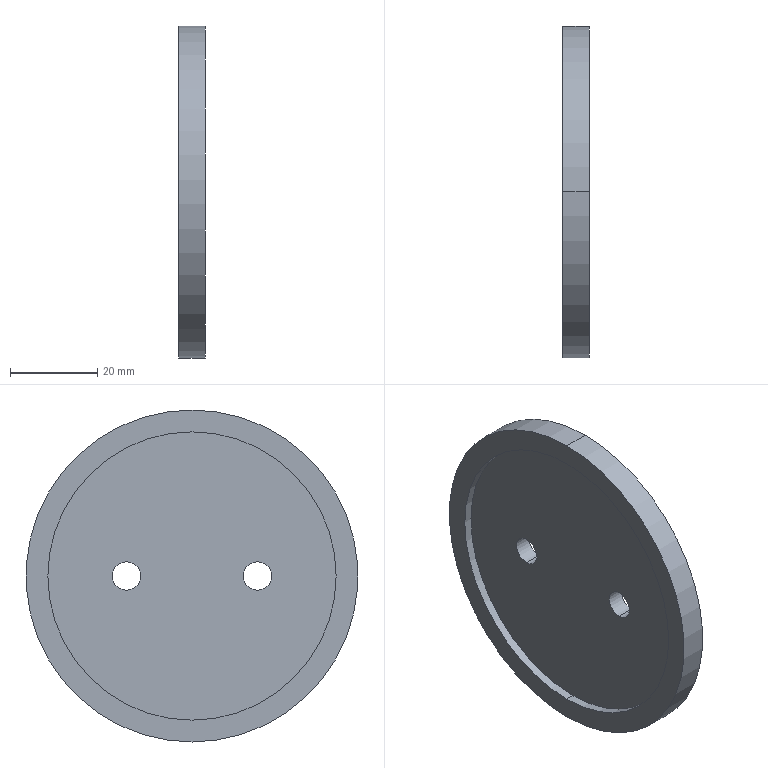Part | SolidWorks | features ICE 1, Revolution 1 | 1 solid | 11 faces | box 6 x 76 x 76 mm | volume 20111 mm3 | cylinder 8 | plane 3 | commonest cylinder face diameters 6.5 x4 66 x2 76 x2
STEP:
#1=CARTESIAN_POINT('',(-4.,-15.,-3.25));
#2=VERTEX_POINT('',#1);
#3=CARTESIAN_POINT('',(-4.,-15.,3.25));
#4=VERTEX_POINT('',#3);
#5=CARTESIAN_POINT('',(-4.,-15.,0.));
#6=DIRECTION('',(-1.,0.,0.));
#7=DIRECTION('',(0.,0.,1.));
#8=AXIS2_PLACEMENT_3D('',#5,#6,#7);
#9=CIRCLE('',#8,3.25);
#10=EDGE_CURVE('',#2,#4,#9,.T.);
#11=ORIENTED_EDGE('',*,*,#10,.T.);
#12=CARTESIAN_POINT('',(0.,-15.,3.25));
#13=VERTEX_POINT('',#12);
#14=CARTESIAN_POINT('',(-6.,-15.,3.25));
#15=DIRECTION('',(1.,0.,0.));
#16=VECTOR('',#15,1000.);
#17=LINE('',#14,#16);
#18=EDGE_CURVE('',#4,#13,#17,.T.);
#19=ORIENTED_EDGE('',*,*,#18,.T.);
#20=CARTESIAN_POINT('',(0.,-15.,-3.25));
#21=VERTEX_POINT('',#20);
#22=CARTESIAN_POINT('',(0.,-15.,0.));
#23=DIRECTION('',(1.,0.,0.));
#24=DIRECTION('',(0.,0.,-1.));
#25=AXIS2_PLACEMENT_3D('',#22,#23,#24);
#26=CIRCLE('',#25,3.25);
#27=EDGE_CURVE('',#13,#21,#26,.T.);
#28=ORIENTED_EDGE('',*,*,#27,.T.);
#29=CARTESIAN_POINT('',(-6.,-15.,-3.25));
#30=DIRECTION('',(1.,0.,0.));
#31=VECTOR('',#30,1000.);
#32=LINE('',#29,#31);
#33=EDGE_CURVE('',#2,#21,#32,.T.);
#34=ORIENTED_EDGE('',*,*,#33,.F.);
#35=EDGE_LOOP('',(#11,#19,#28,#34));
#36=FACE_OUTER_BOUND('',#35,.T.);
#37=CARTESIAN_POINT('',(-6.,-15.,0.));
#38=DIRECTION('',(1.,0.,0.));
#39=DIRECTION('',(0.,0.,-1.));
#40=AXIS2_PLACEMENT_3D('',#37,#38,#39);
#41=CYLINDRICAL_SURFACE('',#40,3.25);
#42=ADVANCED_FACE('',(#36),#41,.F.);
#43=CARTESIAN_POINT('',(-4.,15.,-3.25));
#44=VERTEX_POINT('',#43);
#45=CARTESIAN_POINT('',(-4.,15.,3.25));
#46=VERTEX_POINT('',#45);
#47=CARTESIAN_POINT('',(-4.,15.,0.));
#48=DIRECTION('',(-1.,0.,0.));
#49=DIRECTION('',(0.,0.,1.));
#50=AXIS2_PLACEMENT_3D('',#47,#48,#49);
#51=CIRCLE('',#50,3.25);
#52=EDGE_CURVE('',#44,#46,#51,.T.);
#53=ORIENTED_EDGE('',*,*,#52,.T.);
#54=CARTESIAN_POINT('',(0.,15.,3.25));
#55=VERTEX_POINT('',#54);
#56=CARTESIAN_POINT('',(-6.,15.,3.25));
#57=DIRECTION('',(1.,0.,0.));
#58=VECTOR('',#57,1000.);
#59=LINE('',#56,#58);
#60=EDGE_CURVE('',#46,#55,#59,.T.);
#61=ORIENTED_EDGE('',*,*,#60,.T.);
#62=CARTESIAN_POINT('',(0.,15.,-3.25));
#63=VERTEX_POINT('',#62);
#64=CARTESIAN_POINT('',(0.,15.,0.));
#65=DIRECTION('',(1.,0.,0.));
#66=DIRECTION('',(0.,0.,-1.));
#67=AXIS2_PLACEMENT_3D('',#64,#65,#66);
#68=CIRCLE('',#67,3.25);
#69=EDGE_CURVE('',#55,#63,#68,.T.);
#70=ORIENTED_EDGE('',*,*,#69,.T.);
#71=CARTESIAN_POINT('',(-6.,15.,-3.25));
#72=DIRECTION('',(1.,0.,0.));
#73=VECTOR('',#72,1000.);
#74=LINE('',#71,#73);
#75=EDGE_CURVE('',#44,#63,#74,.T.);
#76=ORIENTED_EDGE('',*,*,#75,.F.);
#77=EDGE_LOOP('',(#53,#61,#70,#76));
#78=FACE_OUTER_BOUND('',#77,.T.);
#79=CARTESIAN_POINT('',(-6.,15.,0.));
#80=DIRECTION('',(1.,0.,0.));
#81=DIRECTION('',(0.,0.,-1.));
#82=AXIS2_PLACEMENT_3D('',#79,#80,#81);
#83=CYLINDRICAL_SURFACE('',#82,3.25);
#84=ADVANCED_FACE('',(#78),#83,.F.);
#85=CARTESIAN_POINT('',(-6.,0.,33.));
#86=VERTEX_POINT('',#85);
#87=CARTESIAN_POINT('',(-6.,0.,-33.));
#88=VERTEX_POINT('',#87);
#89=CARTESIAN_POINT('',(-6.,0.,0.));
#90=DIRECTION('',(1.,0.,0.));
#91=DIRECTION('',(0.,0.,-1.));
#92=AXIS2_PLACEMENT_3D('',#89,#90,#91);
#93=CIRCLE('',#92,33.);
#94=EDGE_CURVE('',#86,#88,#93,.T.);
#95=ORIENTED_EDGE('',*,*,#94,.F.);
#96=CARTESIAN_POINT('',(-4.,0.,33.));
#97=VERTEX_POINT('',#96);
#98=CARTESIAN_POINT('',(0.,0.,33.));
#99=DIRECTION('',(1.,0.,0.));
#100=VECTOR('',#99,1000.);
#101=LINE('',#98,#100);
#102=EDGE_CURVE('',#86,#97,#101,.T.);
#103=ORIENTED_EDGE('',*,*,#102,.T.);
#104=CARTESIAN_POINT('',(-4.,0.,-33.));
#105=VERTEX_POINT('',#104);
#106=CARTESIAN_POINT('',(-4.,0.,0.));
#107=DIRECTION('',(1.,0.,0.));
#108=DIRECTION('',(0.,0.,-1.));
#109=AXIS2_PLACEMENT_3D('',#106,#107,#108);
#110=CIRCLE('',#109,33.);
#111=EDGE_CURVE('',#97,#105,#110,.T.);
#112=ORIENTED_EDGE('',*,*,#111,.T.);
#113=CARTESIAN_POINT('',(0.,0.,-33.));
#114=DIRECTION('',(1.,0.,0.));
#115=VECTOR('',#114,1000.);
#116=LINE('',#113,#115);
#117=EDGE_CURVE('',#88,#105,#116,.T.);
#118=ORIENTED_EDGE('',*,*,#117,.F.);
#119=EDGE_LOOP('',(#95,#103,#112,#118));
#120=FACE_OUTER_BOUND('',#119,.T.);
#121=CARTESIAN_POINT('',(0.,0.,0.));
#122=DIRECTION('',(1.,0.,0.));
#123=DIRECTION('',(0.,0.,-1.));
#124=AXIS2_PLACEMENT_3D('',#121,#122,#123);
#125=CYLINDRICAL_SURFACE('',#124,33.);
#126=ADVANCED_FACE('',(#120),#125,.F.);
#127=CARTESIAN_POINT('',(-6.,0.,-38.));
#128=VERTEX_POINT('',#127);
#129=CARTESIAN_POINT('',(-6.,0.,38.));
#130=VERTEX_POINT('',#129);
#131=CARTESIAN_POINT('',(-6.,0.,0.));
#132=DIRECTION('',(1.,0.,0.));
#133=DIRECTION('',(0.,0.,-1.));
#134=AXIS2_PLACEMENT_3D('',#131,#132,#133);
#135=CIRCLE('',#134,38.);
#136=EDGE_CURVE('',#128,#130,#135,.T.);
#137=ORIENTED_EDGE('',*,*,#136,.T.);
#138=CARTESIAN_POINT('',(0.,0.,38.));
#139=VERTEX_POINT('',#138);
#140=CARTESIAN_POINT('',(0.,0.,38.));
#141=DIRECTION('',(1.,0.,0.));
#142=VECTOR('',#141,1000.);
#143=LINE('',#140,#142);
#144=EDGE_CURVE('',#130,#139,#143,.T.);
#145=ORIENTED_EDGE('',*,*,#144,.T.);
#146=CARTESIAN_POINT('',(0.,0.,-38.));
#147=VERTEX_POINT('',#146);
#148=CARTESIAN_POINT('',(0.,0.,0.));
#149=DIRECTION('',(1.,0.,0.));
#150=DIRECTION('',(0.,0.,-1.));
#151=AXIS2_PLACEMENT_3D('',#148,#149,#150);
#152=CIRCLE('',#151,38.);
#153=EDGE_CURVE('',#147,#139,#152,.T.);
#154=ORIENTED_EDGE('',*,*,#153,.F.);
#155=CARTESIAN_POINT('',(0.,0.,-38.));
#156=DIRECTION('',(1.,0.,0.));
#157=VECTOR('',#156,1000.);
#158=LINE('',#155,#157);
#159=EDGE_CURVE('',#128,#147,#158,.T.);
#160=ORIENTED_EDGE('',*,*,#159,.F.);
#161=EDGE_LOOP('',(#137,#145,#154,#160));
#162=FACE_OUTER_BOUND('',#161,.T.);
#163=CARTESIAN_POINT('',(0.,0.,0.));
#164=DIRECTION('',(1.,0.,0.));
#165=DIRECTION('',(0.,0.,-1.));
#166=AXIS2_PLACEMENT_3D('',#163,#164,#165);
#167=CYLINDRICAL_SURFACE('',#166,38.);
#168=ADVANCED_FACE('',(#162),#167,.T.);
#169=CARTESIAN_POINT('',(0.,-15.,0.));
#170=DIRECTION('',(1.,0.,0.));
#171=DIRECTION('',(0.,0.,-1.));
#172=AXIS2_PLACEMENT_3D('',#169,#170,#171);
#173=CIRCLE('',#172,3.25);
#174=EDGE_CURVE('',#21,#13,#173,.T.);
#175=ORIENTED_EDGE('',*,*,#174,.F.);
#176=ORIENTED_EDGE('',*,*,#27,.F.);
#177=EDGE_LOOP('',(#175,#176));
#178=FACE_BOUND('',#177,.T.);
#179=CARTESIAN_POINT('',(0.,15.,0.));
#180=DIRECTION('',(1.,0.,0.));
#181=DIRECTION('',(0.,0.,-1.));
#182=AXIS2_PLACEMENT_3D('',#179,#180,#181);
#183=CIRCLE('',#182,3.25);
#184=EDGE_CURVE('',#63,#55,#183,.T.);
#185=ORIENTED_EDGE('',*,*,#184,.F.);
#186=ORIENTED_EDGE('',*,*,#69,.F.);
#187=EDGE_LOOP('',(#185,#186));
#188=FACE_BOUND('',#187,.T.);
#189=ORIENTED_EDGE('',*,*,#153,.T.);
#190=CARTESIAN_POINT('',(0.,0.,0.));
#191=DIRECTION('',(1.,0.,0.));
#192=DIRECTION('',(0.,0.,-1.));
#193=AXIS2_PLACEMENT_3D('',#190,#191,#192);
#194=CIRCLE('',#193,38.);
#195=EDGE_CURVE('',#139,#147,#194,.T.);
#196=ORIENTED_EDGE('',*,*,#195,.T.);
#197=EDGE_LOOP('',(#189,#196));
#198=FACE_OUTER_BOUND('',#197,.T.);
#199=CARTESIAN_POINT('',(0.,0.,0.));
#200=DIRECTION('',(1.,0.,0.));
#201=DIRECTION('',(0.,0.,-1.));
#202=AXIS2_PLACEMENT_3D('',#199,#200,#201);
#203=PLANE('',#202);
#204=ADVANCED_FACE('',(#178,#188,#198),#203,.T.);
#205=ORIENTED_EDGE('',*,*,#144,.F.);
#206=CARTESIAN_POINT('',(-6.,0.,0.));
#207=DIRECTION('',(1.,0.,0.));
#208=DIRECTION('',(0.,0.,-1.));
#209=AXIS2_PLACEMENT_3D('',#206,#207,#208);
#210=CIRCLE('',#209,38.);
#211=EDGE_CURVE('',#130,#128,#210,.T.);
#212=ORIENTED_EDGE('',*,*,#211,.T.);
#213=ORIENTED_EDGE('',*,*,#159,.T.);
#214=ORIENTED_EDGE('',*,*,#195,.F.);
#215=EDGE_LOOP('',(#205,#212,#213,#214));
#216=FACE_OUTER_BOUND('',#215,.T.);
#217=CARTESIAN_POINT('',(0.,0.,0.));
#218=DIRECTION('',(1.,0.,0.));
#219=DIRECTION('',(0.,0.,-1.));
#220=AXIS2_PLACEMENT_3D('',#217,#218,#219);
#221=CYLINDRICAL_SURFACE('',#220,38.);
#222=ADVANCED_FACE('',(#216),#221,.T.);
#223=CARTESIAN_POINT('',(-6.,0.,0.));
#224=DIRECTION('',(1.,0.,0.));
#225=DIRECTION('',(0.,0.,-1.));
#226=AXIS2_PLACEMENT_3D('',#223,#224,#225);
#227=CIRCLE('',#226,33.);
#228=EDGE_CURVE('',#88,#86,#227,.T.);
#229=ORIENTED_EDGE('',*,*,#228,.T.);
#230=ORIENTED_EDGE('',*,*,#94,.T.);
#231=EDGE_LOOP('',(#229,#230));
#232=FACE_BOUND('',#231,.T.);
#233=ORIENTED_EDGE('',*,*,#136,.F.);
#234=ORIENTED_EDGE('',*,*,#211,.F.);
#235=EDGE_LOOP('',(#233,#234));
#236=FACE_OUTER_BOUND('',#235,.T.);
#237=CARTESIAN_POINT('',(-6.,38.,0.));
#238=DIRECTION('',(-1.,0.,0.));
#239=DIRECTION('',(0.,0.,1.));
#240=AXIS2_PLACEMENT_3D('',#237,#238,#239);
#241=PLANE('',#240);
#242=ADVANCED_FACE('',(#232,#236),#241,.T.);
#243=ORIENTED_EDGE('',*,*,#102,.F.);
#244=ORIENTED_EDGE('',*,*,#228,.F.);
#245=ORIENTED_EDGE('',*,*,#117,.T.);
#246=CARTESIAN_POINT('',(-4.,0.,0.));
#247=DIRECTION('',(1.,0.,0.));
#248=DIRECTION('',(0.,0.,-1.));
#249=AXIS2_PLACEMENT_3D('',#246,#247,#248);
#250=CIRCLE('',#249,33.);
#251=EDGE_CURVE('',#105,#97,#250,.T.);
#252=ORIENTED_EDGE('',*,*,#251,.T.);
#253=EDGE_LOOP('',(#243,#244,#245,#252));
#254=FACE_OUTER_BOUND('',#253,.T.);
#255=CARTESIAN_POINT('',(0.,0.,0.));
#256=DIRECTION('',(1.,0.,0.));
#257=DIRECTION('',(0.,0.,-1.));
#258=AXIS2_PLACEMENT_3D('',#255,#256,#257);
#259=CYLINDRICAL_SURFACE('',#258,33.);
#260=ADVANCED_FACE('',(#254),#259,.F.);
#261=ORIENTED_EDGE('',*,*,#10,.F.);
#262=CARTESIAN_POINT('',(-4.,-15.,0.));
#263=DIRECTION('',(-1.,0.,0.));
#264=DIRECTION('',(0.,0.,1.));
#265=AXIS2_PLACEMENT_3D('',#262,#263,#264);
#266=CIRCLE('',#265,3.25);
#267=EDGE_CURVE('',#4,#2,#266,.T.);
#268=ORIENTED_EDGE('',*,*,#267,.F.);
#269=EDGE_LOOP('',(#261,#268));
#270=FACE_BOUND('',#269,.T.);
#271=ORIENTED_EDGE('',*,*,#52,.F.);
#272=CARTESIAN_POINT('',(-4.,15.,0.));
#273=DIRECTION('',(-1.,0.,0.));
#274=DIRECTION('',(0.,0.,1.));
#275=AXIS2_PLACEMENT_3D('',#272,#273,#274);
#276=CIRCLE('',#275,3.25);
#277=EDGE_CURVE('',#46,#44,#276,.T.);
#278=ORIENTED_EDGE('',*,*,#277,.F.);
#279=EDGE_LOOP('',(#271,#278));
#280=FACE_BOUND('',#279,.T.);
#281=ORIENTED_EDGE('',*,*,#251,.F.);
#282=ORIENTED_EDGE('',*,*,#111,.F.);
#283=EDGE_LOOP('',(#281,#282));
#284=FACE_OUTER_BOUND('',#283,.T.);
#285=CARTESIAN_POINT('',(-4.,33.,0.));
#286=DIRECTION('',(-1.,0.,0.));
#287=DIRECTION('',(0.,0.,1.));
#288=AXIS2_PLACEMENT_3D('',#285,#286,#287);
#289=PLANE('',#288);
#290=ADVANCED_FACE('',(#270,#280,#284),#289,.T.);
#291=ORIENTED_EDGE('',*,*,#60,.F.);
#292=ORIENTED_EDGE('',*,*,#277,.T.);
#293=ORIENTED_EDGE('',*,*,#75,.T.);
#294=ORIENTED_EDGE('',*,*,#184,.T.);
#295=EDGE_LOOP('',(#291,#292,#293,#294));
#296=FACE_OUTER_BOUND('',#295,.T.);
#297=CARTESIAN_POINT('',(-6.,15.,0.));
#298=DIRECTION('',(1.,0.,0.));
#299=DIRECTION('',(0.,0.,-1.));
#300=AXIS2_PLACEMENT_3D('',#297,#298,#299);
#301=CYLINDRICAL_SURFACE('',#300,3.25);
#302=ADVANCED_FACE('',(#296),#301,.F.);
#303=ORIENTED_EDGE('',*,*,#18,.F.);
#304=ORIENTED_EDGE('',*,*,#267,.T.);
#305=ORIENTED_EDGE('',*,*,#33,.T.);
#306=ORIENTED_EDGE('',*,*,#174,.T.);
#307=EDGE_LOOP('',(#303,#304,#305,#306));
#308=FACE_OUTER_BOUND('',#307,.T.);
#309=CARTESIAN_POINT('',(-6.,-15.,0.));
#310=DIRECTION('',(1.,0.,0.));
#311=DIRECTION('',(0.,0.,-1.));
#312=AXIS2_PLACEMENT_3D('',#309,#310,#311);
#313=CYLINDRICAL_SURFACE('',#312,3.25);
#314=ADVANCED_FACE('',(#308),#313,.F.);
#315=CLOSED_SHELL('',(#42,#84,#126,#168,#204,#222,#242,#260,#290,#302,#314));
#316=MANIFOLD_SOLID_BREP('',#315);
#317=CARTESIAN_POINT('',(0.,0.,0.));
#318=DIRECTION('',(0.,0.,1.));
#319=DIRECTION('',(1.,0.,0.));
#320=AXIS2_PLACEMENT_3D('',#317,#318,#319);
#321=(LENGTH_UNIT()NAMED_UNIT(*)SI_UNIT(.MILLI.,.METRE.));
#322=UNCERTAINTY_MEASURE_WITH_UNIT(LENGTH_MEASURE(0.00001),#321,'','');
#323=(NAMED_UNIT(*)PLANE_ANGLE_UNIT()SI_UNIT($,.RADIAN.));
#324=(NAMED_UNIT(*)SI_UNIT($,.STERADIAN.)SOLID_ANGLE_UNIT());
#325=(GEOMETRIC_REPRESENTATION_CONTEXT(3)GLOBAL_UNCERTAINTY_ASSIGNED_CONTEXT((#322))GLOBAL_UNIT_ASSIGNED_CONTEXT((#321,#323,#324))REPRESENTATION_CONTEXT('',''));
#326=ADVANCED_BREP_SHAPE_REPRESENTATION('',(#316,#320),#325);